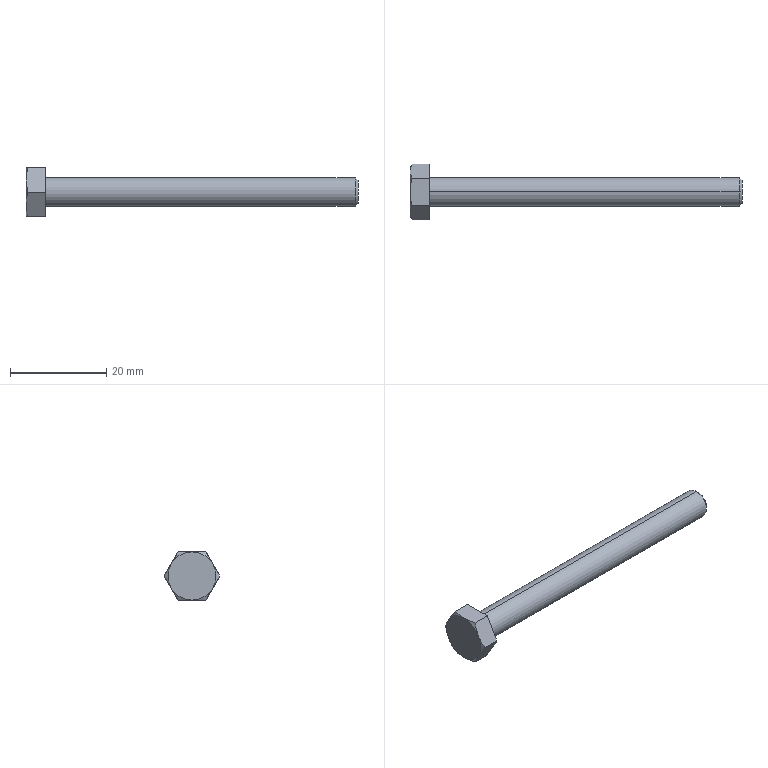Part | STEP file | 0243_314_RCB6-65 | 1 solid | 19 faces | box 69 x 11.547 x 10 mm | volume 2180 mm3 | plane 9 | cone 8 | cylinder 2 | commonest cylinder face diameters 6 x2